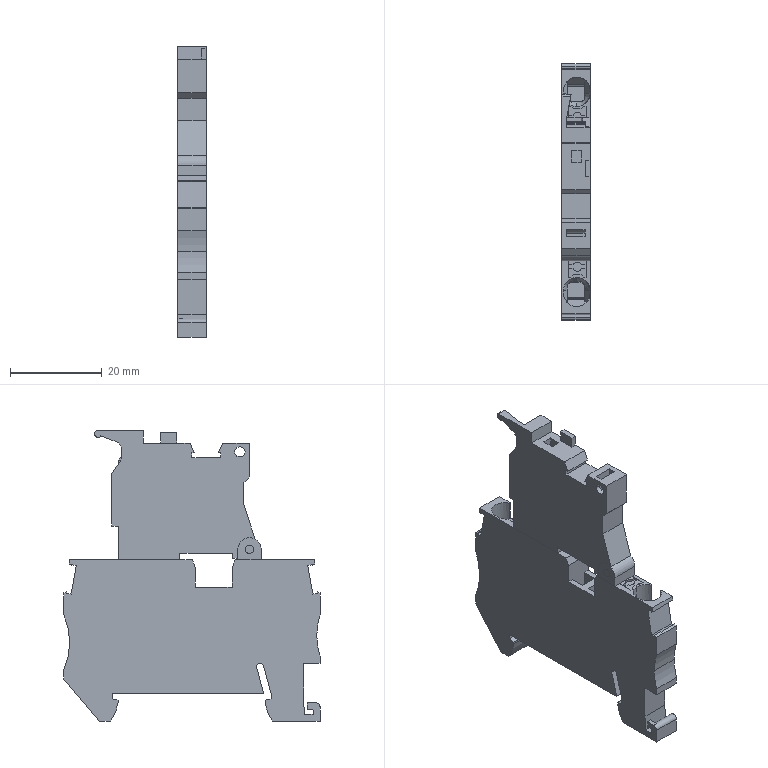Part | STEP file | Fuse terminal block PT4-HESILED24(5x20)-3211903 | 1 solid | 221 faces | box 6.15 x 55.9 x 63.38 mm | volume 12999 mm3 | plane 180 | cylinder 33 | cone 4 | torus 4 | commonest cylinder face diameters 2 x8 5.8 x6 1.4 x4 30 x3 1.8 x2 2.25 x2